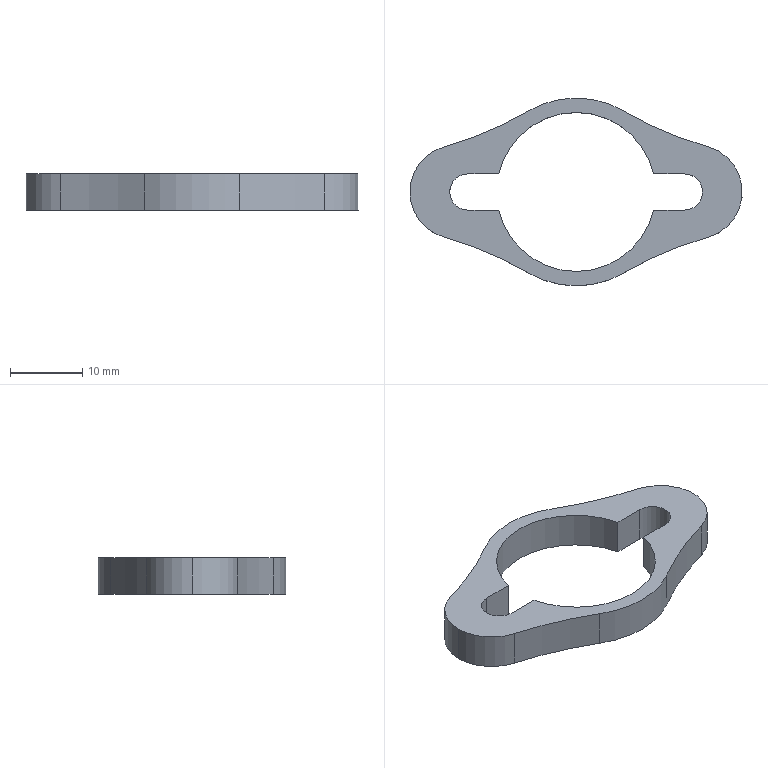Part | SolidWorks | features BaseBody 1 | 1 solid | 20 faces | box 46 x 26 x 5 mm | volume 1841 mm3 | cylinder 14 | plane 6 | commonest cylinder face diameters 100 x4 5 x3 13 x3 22 x2 26 x2
STEP:
#1=CARTESIAN_POINT('',(465.537,40.215,0.366));
#2=VERTEX_POINT('',#1);
#3=CARTESIAN_POINT('',(463.037,37.715,0.366));
#4=VERTEX_POINT('',#3);
#5=CARTESIAN_POINT('',(465.537,37.715,0.366));
#6=DIRECTION('',(-0.000000013,0.,1.));
#7=DIRECTION('',(-1.,0.,-0.000000013));
#8=AXIS2_PLACEMENT_3D('',#5,#6,#7);
#9=CIRCLE('',#8,2.5);
#10=EDGE_CURVE('',#2,#4,#9,.T.);
#11=ORIENTED_EDGE('',*,*,#10,.T.);
#12=CARTESIAN_POINT('',(463.037,37.715,-4.634));
#13=VERTEX_POINT('',#12);
#14=CARTESIAN_POINT('',(463.037,37.715,0.366));
#15=DIRECTION('',(0.000000013,0.,-1.));
#16=VECTOR('',#15,1000.);
#17=LINE('',#14,#16);
#18=EDGE_CURVE('',#4,#13,#17,.T.);
#19=ORIENTED_EDGE('',*,*,#18,.T.);
#20=CARTESIAN_POINT('',(465.537,40.215,-4.634));
#21=VERTEX_POINT('',#20);
#22=CARTESIAN_POINT('',(465.537,37.715,-4.634));
#23=DIRECTION('',(0.000000013,0.,-1.));
#24=DIRECTION('',(-1.,0.,-0.000000013));
#25=AXIS2_PLACEMENT_3D('',#22,#23,#24);
#26=CIRCLE('',#25,2.5);
#27=EDGE_CURVE('',#13,#21,#26,.T.);
#28=ORIENTED_EDGE('',*,*,#27,.T.);
#29=CARTESIAN_POINT('',(465.537,40.215,-2.134));
#30=DIRECTION('',(0.000000013,0.,-1.));
#31=VECTOR('',#30,1000.);
#32=LINE('',#29,#31);
#33=EDGE_CURVE('',#2,#21,#32,.T.);
#34=ORIENTED_EDGE('',*,*,#33,.F.);
#35=EDGE_LOOP('',(#11,#19,#28,#34));
#36=FACE_OUTER_BOUND('',#35,.T.);
#37=CARTESIAN_POINT('',(465.537,37.715,0.366));
#38=DIRECTION('',(0.000000013,0.,-1.));
#39=DIRECTION('',(-1.,0.,-0.000000013));
#40=AXIS2_PLACEMENT_3D('',#37,#38,#39);
#41=CYLINDRICAL_SURFACE('',#40,2.5);
#42=ADVANCED_FACE('',(#36),#41,.F.);
#43=CARTESIAN_POINT('',(462.278,31.457,0.366));
#44=VERTEX_POINT('',#43);
#45=CARTESIAN_POINT('',(457.537,37.715,0.366));
#46=VERTEX_POINT('',#45);
#47=CARTESIAN_POINT('',(464.037,37.715,0.366));
#48=DIRECTION('',(0.000000013,0.,-1.));
#49=DIRECTION('',(-1.,0.,-0.000000013));
#50=AXIS2_PLACEMENT_3D('',#47,#48,#49);
#51=CIRCLE('',#50,6.5);
#52=EDGE_CURVE('',#44,#46,#51,.T.);
#53=ORIENTED_EDGE('',*,*,#52,.T.);
#54=CARTESIAN_POINT('',(457.537,37.715,-4.634));
#55=VERTEX_POINT('',#54);
#56=CARTESIAN_POINT('',(457.537,37.715,0.366));
#57=DIRECTION('',(0.000000013,0.,-1.));
#58=VECTOR('',#57,1000.);
#59=LINE('',#56,#58);
#60=EDGE_CURVE('',#46,#55,#59,.T.);
#61=ORIENTED_EDGE('',*,*,#60,.T.);
#62=CARTESIAN_POINT('',(462.278,31.457,-4.634));
#63=VERTEX_POINT('',#62);
#64=CARTESIAN_POINT('',(464.037,37.715,-4.634));
#65=DIRECTION('',(0.000000013,0.,-1.));
#66=DIRECTION('',(-1.,0.,-0.000000013));
#67=AXIS2_PLACEMENT_3D('',#64,#65,#66);
#68=CIRCLE('',#67,6.5);
#69=EDGE_CURVE('',#63,#55,#68,.T.);
#70=ORIENTED_EDGE('',*,*,#69,.F.);
#71=CARTESIAN_POINT('',(462.278,31.457,-2.134));
#72=DIRECTION('',(0.000000013,0.,-1.));
#73=VECTOR('',#72,1000.);
#74=LINE('',#71,#73);
#75=EDGE_CURVE('',#44,#63,#74,.T.);
#76=ORIENTED_EDGE('',*,*,#75,.F.);
#77=EDGE_LOOP('',(#53,#61,#70,#76));
#78=FACE_OUTER_BOUND('',#77,.T.);
#79=CARTESIAN_POINT('',(464.037,37.715,0.366));
#80=DIRECTION('',(0.000000013,0.,-1.));
#81=DIRECTION('',(-1.,0.,-0.000000013));
#82=AXIS2_PLACEMENT_3D('',#79,#80,#81);
#83=CYLINDRICAL_SURFACE('',#82,6.5);
#84=ADVANCED_FACE('',(#78),#83,.T.);
#85=CARTESIAN_POINT('',(491.249,40.215,0.366));
#86=VERTEX_POINT('',#85);
#87=CARTESIAN_POINT('',(469.825,40.215,0.366));
#88=VERTEX_POINT('',#87);
#89=CARTESIAN_POINT('',(480.537,37.715,0.366));
#90=DIRECTION('',(-0.000000013,0.,1.));
#91=DIRECTION('',(-1.,0.,-0.000000013));
#92=AXIS2_PLACEMENT_3D('',#89,#90,#91);
#93=CIRCLE('',#92,11.);
#94=EDGE_CURVE('',#86,#88,#93,.T.);
#95=ORIENTED_EDGE('',*,*,#94,.F.);
#96=CARTESIAN_POINT('',(495.537,40.215,0.366));
#97=VERTEX_POINT('',#96);
#98=CARTESIAN_POINT('',(480.537,40.215,0.366));
#99=DIRECTION('',(-1.,0.,-0.000000013));
#100=VECTOR('',#99,1000.);
#101=LINE('',#98,#100);
#102=EDGE_CURVE('',#97,#86,#101,.T.);
#103=ORIENTED_EDGE('',*,*,#102,.F.);
#104=CARTESIAN_POINT('',(495.537,35.215,0.366));
#105=VERTEX_POINT('',#104);
#106=CARTESIAN_POINT('',(495.537,37.715,0.366));
#107=DIRECTION('',(-0.000000013,0.,1.));
#108=DIRECTION('',(-1.,0.,-0.000000013));
#109=AXIS2_PLACEMENT_3D('',#106,#107,#108);
#110=CIRCLE('',#109,2.5);
#111=EDGE_CURVE('',#105,#97,#110,.T.);
#112=ORIENTED_EDGE('',*,*,#111,.F.);
#113=CARTESIAN_POINT('',(491.249,35.215,0.366));
#114=VERTEX_POINT('',#113);
#115=CARTESIAN_POINT('',(480.537,35.215,0.366));
#116=DIRECTION('',(1.,0.,0.000000013));
#117=VECTOR('',#116,1000.);
#118=LINE('',#115,#117);
#119=EDGE_CURVE('',#114,#105,#118,.T.);
#120=ORIENTED_EDGE('',*,*,#119,.F.);
#121=CARTESIAN_POINT('',(469.825,35.215,0.366));
#122=VERTEX_POINT('',#121);
#123=CARTESIAN_POINT('',(480.537,37.715,0.366));
#124=DIRECTION('',(-0.000000013,0.,1.));
#125=DIRECTION('',(-1.,0.,-0.000000013));
#126=AXIS2_PLACEMENT_3D('',#123,#124,#125);
#127=CIRCLE('',#126,11.);
#128=EDGE_CURVE('',#122,#114,#127,.T.);
#129=ORIENTED_EDGE('',*,*,#128,.F.);
#130=CARTESIAN_POINT('',(465.537,35.215,0.366));
#131=VERTEX_POINT('',#130);
#132=CARTESIAN_POINT('',(480.537,35.215,0.366));
#133=DIRECTION('',(1.,0.,0.000000013));
#134=VECTOR('',#133,1000.);
#135=LINE('',#132,#134);
#136=EDGE_CURVE('',#131,#122,#135,.T.);
#137=ORIENTED_EDGE('',*,*,#136,.F.);
#138=CARTESIAN_POINT('',(465.537,37.715,0.366));
#139=DIRECTION('',(-0.000000013,0.,1.));
#140=DIRECTION('',(-1.,0.,-0.000000013));
#141=AXIS2_PLACEMENT_3D('',#138,#139,#140);
#142=CIRCLE('',#141,2.5);
#143=EDGE_CURVE('',#4,#131,#142,.T.);
#144=ORIENTED_EDGE('',*,*,#143,.F.);
#145=ORIENTED_EDGE('',*,*,#10,.F.);
#146=CARTESIAN_POINT('',(480.537,40.215,0.366));
#147=DIRECTION('',(-1.,0.,-0.000000013));
#148=VECTOR('',#147,1000.);
#149=LINE('',#146,#148);
#150=EDGE_CURVE('',#88,#2,#149,.T.);
#151=ORIENTED_EDGE('',*,*,#150,.F.);
#152=EDGE_LOOP('',(#95,#103,#112,#120,#129,#137,#144,#145,#151));
#153=FACE_BOUND('',#152,.T.);
#154=CARTESIAN_POINT('',(462.278,43.972,0.366));
#155=VERTEX_POINT('',#154);
#156=CARTESIAN_POINT('',(473.977,48.939,0.366));
#157=VERTEX_POINT('',#156);
#158=CARTESIAN_POINT('',(448.749,92.107,0.366));
#159=DIRECTION('',(-0.000000013,0.,1.));
#160=DIRECTION('',(-1.,0.,-0.000000013));
#161=AXIS2_PLACEMENT_3D('',#158,#159,#160);
#162=CIRCLE('',#161,50.);
#163=EDGE_CURVE('',#155,#157,#162,.T.);
#164=ORIENTED_EDGE('',*,*,#163,.F.);
#165=CARTESIAN_POINT('',(464.037,37.715,0.366));
#166=DIRECTION('',(0.000000013,0.,-1.));
#167=DIRECTION('',(-1.,0.,-0.000000013));
#168=AXIS2_PLACEMENT_3D('',#165,#166,#167);
#169=CIRCLE('',#168,6.5);
#170=EDGE_CURVE('',#46,#155,#169,.T.);
#171=ORIENTED_EDGE('',*,*,#170,.F.);
#172=ORIENTED_EDGE('',*,*,#52,.F.);
#173=CARTESIAN_POINT('',(473.977,26.491,0.366));
#174=VERTEX_POINT('',#173);
#175=CARTESIAN_POINT('',(448.749,-16.678,0.366));
#176=DIRECTION('',(-0.000000013,0.,1.));
#177=DIRECTION('',(-1.,0.,-0.000000013));
#178=AXIS2_PLACEMENT_3D('',#175,#176,#177);
#179=CIRCLE('',#178,50.);
#180=EDGE_CURVE('',#174,#44,#179,.T.);
#181=ORIENTED_EDGE('',*,*,#180,.F.);
#182=CARTESIAN_POINT('',(487.096,26.491,0.366));
#183=VERTEX_POINT('',#182);
#184=CARTESIAN_POINT('',(480.537,37.715,0.366));
#185=DIRECTION('',(0.000000013,0.,-1.));
#186=DIRECTION('',(-1.,0.,-0.000000013));
#187=AXIS2_PLACEMENT_3D('',#184,#185,#186);
#188=CIRCLE('',#187,13.);
#189=EDGE_CURVE('',#183,#174,#188,.T.);
#190=ORIENTED_EDGE('',*,*,#189,.F.);
#191=CARTESIAN_POINT('',(498.796,31.457,0.366));
#192=VERTEX_POINT('',#191);
#193=CARTESIAN_POINT('',(512.325,-16.678,0.366));
#194=DIRECTION('',(-0.000000013,0.,1.));
#195=DIRECTION('',(-1.,0.,-0.000000013));
#196=AXIS2_PLACEMENT_3D('',#193,#194,#195);
#197=CIRCLE('',#196,50.);
#198=EDGE_CURVE('',#192,#183,#197,.T.);
#199=ORIENTED_EDGE('',*,*,#198,.F.);
#200=CARTESIAN_POINT('',(498.796,43.972,0.366));
#201=VERTEX_POINT('',#200);
#202=CARTESIAN_POINT('',(497.037,37.715,0.366));
#203=DIRECTION('',(0.000000013,0.,-1.));
#204=DIRECTION('',(-1.,0.,-0.000000013));
#205=AXIS2_PLACEMENT_3D('',#202,#203,#204);
#206=CIRCLE('',#205,6.5);
#207=EDGE_CURVE('',#201,#192,#206,.T.);
#208=ORIENTED_EDGE('',*,*,#207,.F.);
#209=CARTESIAN_POINT('',(487.096,48.939,0.366));
#210=VERTEX_POINT('',#209);
#211=CARTESIAN_POINT('',(512.325,92.107,0.366));
#212=DIRECTION('',(-0.000000013,0.,1.));
#213=DIRECTION('',(-1.,0.,-0.000000013));
#214=AXIS2_PLACEMENT_3D('',#211,#212,#213);
#215=CIRCLE('',#214,50.);
#216=EDGE_CURVE('',#210,#201,#215,.T.);
#217=ORIENTED_EDGE('',*,*,#216,.F.);
#218=CARTESIAN_POINT('',(480.537,37.715,0.366));
#219=DIRECTION('',(0.000000013,0.,-1.));
#220=DIRECTION('',(-1.,0.,-0.000000013));
#221=AXIS2_PLACEMENT_3D('',#218,#219,#220);
#222=CIRCLE('',#221,13.);
#223=EDGE_CURVE('',#157,#210,#222,.T.);
#224=ORIENTED_EDGE('',*,*,#223,.F.);
#225=EDGE_LOOP('',(#164,#171,#172,#181,#190,#199,#208,#217,#224));
#226=FACE_OUTER_BOUND('',#225,.T.);
#227=CARTESIAN_POINT('',(504.464,24.183,0.366));
#228=DIRECTION('',(0.000000013,0.,-1.));
#229=DIRECTION('',(-1.,0.,-0.000000013));
#230=AXIS2_PLACEMENT_3D('',#227,#228,#229);
#231=PLANE('',#230);
#232=ADVANCED_FACE('',(#153,#226),#231,.F.);
#233=CARTESIAN_POINT('',(469.825,40.215,-4.634));
#234=VERTEX_POINT('',#233);
#235=CARTESIAN_POINT('',(467.681,40.215,-4.634));
#236=DIRECTION('',(1.,0.,0.000000013));
#237=VECTOR('',#236,1000.);
#238=LINE('',#235,#237);
#239=EDGE_CURVE('',#21,#234,#238,.T.);
#240=ORIENTED_EDGE('',*,*,#239,.T.);
#241=CARTESIAN_POINT('',(469.825,40.215,-2.134));
#242=DIRECTION('',(-0.000000013,0.,1.));
#243=VECTOR('',#242,1000.);
#244=LINE('',#241,#243);
#245=EDGE_CURVE('',#234,#88,#244,.T.);
#246=ORIENTED_EDGE('',*,*,#245,.T.);
#247=ORIENTED_EDGE('',*,*,#150,.T.);
#248=ORIENTED_EDGE('',*,*,#33,.T.);
#249=EDGE_LOOP('',(#240,#246,#247,#248));
#250=FACE_OUTER_BOUND('',#249,.T.);
#251=CARTESIAN_POINT('',(469.91,40.215,0.466));
#252=DIRECTION('',(0.,-1.,0.));
#253=DIRECTION('',(-1.,0.,-0.000000013));
#254=AXIS2_PLACEMENT_3D('',#251,#252,#253);
#255=PLANE('',#254);
#256=ADVANCED_FACE('',(#250),#255,.T.);
#257=CARTESIAN_POINT('',(491.249,40.215,-4.634));
#258=VERTEX_POINT('',#257);
#259=CARTESIAN_POINT('',(480.537,37.715,-4.634));
#260=DIRECTION('',(0.000000013,0.,-1.));
#261=DIRECTION('',(-1.,0.,-0.000000013));
#262=AXIS2_PLACEMENT_3D('',#259,#260,#261);
#263=CIRCLE('',#262,11.);
#264=EDGE_CURVE('',#234,#258,#263,.T.);
#265=ORIENTED_EDGE('',*,*,#264,.T.);
#266=CARTESIAN_POINT('',(491.249,40.215,-2.134));
#267=DIRECTION('',(-0.000000013,0.,1.));
#268=VECTOR('',#267,1000.);
#269=LINE('',#266,#268);
#270=EDGE_CURVE('',#258,#86,#269,.T.);
#271=ORIENTED_EDGE('',*,*,#270,.T.);
#272=ORIENTED_EDGE('',*,*,#94,.T.);
#273=ORIENTED_EDGE('',*,*,#245,.F.);
#274=EDGE_LOOP('',(#265,#271,#272,#273));
#275=FACE_OUTER_BOUND('',#274,.T.);
#276=CARTESIAN_POINT('',(480.537,37.715,0.366));
#277=DIRECTION('',(0.000000013,0.,-1.));
#278=DIRECTION('',(-1.,0.,-0.000000013));
#279=AXIS2_PLACEMENT_3D('',#276,#277,#278);
#280=CYLINDRICAL_SURFACE('',#279,11.);
#281=ADVANCED_FACE('',(#275),#280,.F.);
#282=CARTESIAN_POINT('',(495.537,40.215,-4.634));
#283=VERTEX_POINT('',#282);
#284=CARTESIAN_POINT('',(493.393,40.215,-4.634));
#285=DIRECTION('',(1.,0.,0.000000013));
#286=VECTOR('',#285,1000.);
#287=LINE('',#284,#286);
#288=EDGE_CURVE('',#258,#283,#287,.T.);
#289=ORIENTED_EDGE('',*,*,#288,.T.);
#290=CARTESIAN_POINT('',(495.537,40.215,-2.134));
#291=DIRECTION('',(-0.000000013,0.,1.));
#292=VECTOR('',#291,1000.);
#293=LINE('',#290,#292);
#294=EDGE_CURVE('',#283,#97,#293,.T.);
#295=ORIENTED_EDGE('',*,*,#294,.T.);
#296=ORIENTED_EDGE('',*,*,#102,.T.);
#297=ORIENTED_EDGE('',*,*,#270,.F.);
#298=EDGE_LOOP('',(#289,#295,#296,#297));
#299=FACE_OUTER_BOUND('',#298,.T.);
#300=CARTESIAN_POINT('',(495.623,40.215,0.466));
#301=DIRECTION('',(0.,-1.,0.));
#302=DIRECTION('',(-1.,0.,-0.000000013));
#303=AXIS2_PLACEMENT_3D('',#300,#301,#302);
#304=PLANE('',#303);
#305=ADVANCED_FACE('',(#299),#304,.T.);
#306=ORIENTED_EDGE('',*,*,#294,.F.);
#307=CARTESIAN_POINT('',(495.537,35.215,-4.634));
#308=VERTEX_POINT('',#307);
#309=CARTESIAN_POINT('',(495.537,37.715,-4.634));
#310=DIRECTION('',(0.000000013,0.,-1.));
#311=DIRECTION('',(-1.,0.,-0.000000013));
#312=AXIS2_PLACEMENT_3D('',#309,#310,#311);
#313=CIRCLE('',#312,2.5);
#314=EDGE_CURVE('',#283,#308,#313,.T.);
#315=ORIENTED_EDGE('',*,*,#314,.T.);
#316=CARTESIAN_POINT('',(495.537,35.215,-2.134));
#317=DIRECTION('',(-0.000000013,0.,1.));
#318=VECTOR('',#317,1000.);
#319=LINE('',#316,#318);
#320=EDGE_CURVE('',#308,#105,#319,.T.);
#321=ORIENTED_EDGE('',*,*,#320,.T.);
#322=ORIENTED_EDGE('',*,*,#111,.T.);
#323=EDGE_LOOP('',(#306,#315,#321,#322));
#324=FACE_OUTER_BOUND('',#323,.T.);
#325=CARTESIAN_POINT('',(495.537,37.715,0.366));
#326=DIRECTION('',(0.000000013,0.,-1.));
#327=DIRECTION('',(-1.,0.,-0.000000013));
#328=AXIS2_PLACEMENT_3D('',#325,#326,#327);
#329=CYLINDRICAL_SURFACE('',#328,2.5);
#330=ADVANCED_FACE('',(#324),#329,.F.);
#331=CARTESIAN_POINT('',(491.249,35.215,-4.634));
#332=VERTEX_POINT('',#331);
#333=CARTESIAN_POINT('',(493.393,35.215,-4.634));
#334=DIRECTION('',(-1.,0.,-0.000000013));
#335=VECTOR('',#334,1000.);
#336=LINE('',#333,#335);
#337=EDGE_CURVE('',#308,#332,#336,.T.);
#338=ORIENTED_EDGE('',*,*,#337,.T.);
#339=CARTESIAN_POINT('',(491.249,35.215,-2.134));
#340=DIRECTION('',(-0.000000013,0.,1.));
#341=VECTOR('',#340,1000.);
#342=LINE('',#339,#341);
#343=EDGE_CURVE('',#332,#114,#342,.T.);
#344=ORIENTED_EDGE('',*,*,#343,.T.);
#345=ORIENTED_EDGE('',*,*,#119,.T.);
#346=ORIENTED_EDGE('',*,*,#320,.F.);
#347=EDGE_LOOP('',(#338,#344,#345,#346));
#348=FACE_OUTER_BOUND('',#347,.T.);
#349=CARTESIAN_POINT('',(491.163,35.215,0.466));
#350=DIRECTION('',(0.,1.,0.));
#351=DIRECTION('',(1.,0.,0.000000013));
#352=AXIS2_PLACEMENT_3D('',#349,#350,#351);
#353=PLANE('',#352);
#354=ADVANCED_FACE('',(#348),#353,.T.);
#355=CARTESIAN_POINT('',(469.825,35.215,-4.634));
#356=VERTEX_POINT('',#355);
#357=CARTESIAN_POINT('',(480.537,37.715,-4.634));
#358=DIRECTION('',(0.000000013,0.,-1.));
#359=DIRECTION('',(-1.,0.,-0.000000013));
#360=AXIS2_PLACEMENT_3D('',#357,#358,#359);
#361=CIRCLE('',#360,11.);
#362=EDGE_CURVE('',#332,#356,#361,.T.);
#363=ORIENTED_EDGE('',*,*,#362,.T.);
#364=CARTESIAN_POINT('',(469.825,35.215,-2.134));
#365=DIRECTION('',(-0.000000013,0.,1.));
#366=VECTOR('',#365,1000.);
#367=LINE('',#364,#366);
#368=EDGE_CURVE('',#356,#122,#367,.T.);
#369=ORIENTED_EDGE('',*,*,#368,.T.);
#370=ORIENTED_EDGE('',*,*,#128,.T.);
#371=ORIENTED_EDGE('',*,*,#343,.F.);
#372=EDGE_LOOP('',(#363,#369,#370,#371));
#373=FACE_OUTER_BOUND('',#372,.T.);
#374=CARTESIAN_POINT('',(480.537,37.715,0.366));
#375=DIRECTION('',(0.000000013,0.,-1.));
#376=DIRECTION('',(-1.,0.,-0.000000013));
#377=AXIS2_PLACEMENT_3D('',#374,#375,#376);
#378=CYLINDRICAL_SURFACE('',#377,11.);
#379=ADVANCED_FACE('',(#373),#378,.F.);
#380=CARTESIAN_POINT('',(465.537,35.215,-4.634));
#381=VERTEX_POINT('',#380);
#382=CARTESIAN_POINT('',(467.681,35.215,-4.634));
#383=DIRECTION('',(-1.,0.,-0.000000013));
#384=VECTOR('',#383,1000.);
#385=LINE('',#382,#384);
#386=EDGE_CURVE('',#356,#381,#385,.T.);
#387=ORIENTED_EDGE('',*,*,#386,.T.);
#388=CARTESIAN_POINT('',(465.537,35.215,-2.134));
#389=DIRECTION('',(-0.000000013,0.,1.));
#390=VECTOR('',#389,1000.);
#391=LINE('',#388,#390);
#392=EDGE_CURVE('',#381,#131,#391,.T.);
#393=ORIENTED_EDGE('',*,*,#392,.T.);
#394=ORIENTED_EDGE('',*,*,#136,.T.);
#395=ORIENTED_EDGE('',*,*,#368,.F.);
#396=EDGE_LOOP('',(#387,#393,#394,#395));
#397=FACE_OUTER_BOUND('',#396,.T.);
#398=CARTESIAN_POINT('',(465.451,35.215,0.466));
#399=DIRECTION('',(0.,1.,0.));
#400=DIRECTION('',(1.,0.,0.000000013));
#401=AXIS2_PLACEMENT_3D('',#398,#399,#400);
#402=PLANE('',#401);
#403=ADVANCED_FACE('',(#397),#402,.T.);
#404=ORIENTED_EDGE('',*,*,#18,.F.);
#405=ORIENTED_EDGE('',*,*,#143,.T.);
#406=ORIENTED_EDGE('',*,*,#392,.F.);
#407=CARTESIAN_POINT('',(465.537,37.715,-4.634));
#408=DIRECTION('',(0.000000013,0.,-1.));
#409=DIRECTION('',(-1.,0.,-0.000000013));
#410=AXIS2_PLACEMENT_3D('',#407,#408,#409);
#411=CIRCLE('',#410,2.5);
#412=EDGE_CURVE('',#381,#13,#411,.T.);
#413=ORIENTED_EDGE('',*,*,#412,.T.);
#414=EDGE_LOOP('',(#404,#405,#406,#413));
#415=FACE_OUTER_BOUND('',#414,.T.);
#416=CARTESIAN_POINT('',(465.537,37.715,0.366));
#417=DIRECTION('',(0.000000013,0.,-1.));
#418=DIRECTION('',(-1.,0.,-0.000000013));
#419=AXIS2_PLACEMENT_3D('',#416,#417,#418);
#420=CYLINDRICAL_SURFACE('',#419,2.5);
#421=ADVANCED_FACE('',(#415),#420,.F.);
#422=CARTESIAN_POINT('',(487.096,48.939,-4.634));
#423=VERTEX_POINT('',#422);
#424=CARTESIAN_POINT('',(487.096,48.939,-2.134));
#425=DIRECTION('',(-0.000000013,0.,1.));
#426=VECTOR('',#425,1000.);
#427=LINE('',#424,#426);
#428=EDGE_CURVE('',#423,#210,#427,.T.);
#429=ORIENTED_EDGE('',*,*,#428,.F.);
#430=CARTESIAN_POINT('',(473.977,48.939,-4.634));
#431=VERTEX_POINT('',#430);
#432=CARTESIAN_POINT('',(480.537,37.715,-4.634));
#433=DIRECTION('',(0.000000013,0.,-1.));
#434=DIRECTION('',(-1.,0.,-0.000000013));
#435=AXIS2_PLACEMENT_3D('',#432,#433,#434);
#436=CIRCLE('',#435,13.);
#437=EDGE_CURVE('',#431,#423,#436,.T.);
#438=ORIENTED_EDGE('',*,*,#437,.F.);
#439=CARTESIAN_POINT('',(473.977,48.939,-2.134));
#440=DIRECTION('',(0.000000013,0.,-1.));
#441=VECTOR('',#440,1000.);
#442=LINE('',#439,#441);
#443=EDGE_CURVE('',#157,#431,#442,.T.);
#444=ORIENTED_EDGE('',*,*,#443,.F.);
#445=ORIENTED_EDGE('',*,*,#223,.T.);
#446=EDGE_LOOP('',(#429,#438,#444,#445));
#447=FACE_OUTER_BOUND('',#446,.T.);
#448=CARTESIAN_POINT('',(480.537,37.715,0.366));
#449=DIRECTION('',(0.000000013,0.,-1.));
#450=DIRECTION('',(-1.,0.,-0.000000013));
#451=AXIS2_PLACEMENT_3D('',#448,#449,#450);
#452=CYLINDRICAL_SURFACE('',#451,13.);
#453=ADVANCED_FACE('',(#447),#452,.T.);
#454=CARTESIAN_POINT('',(462.278,43.972,-4.634));
#455=VERTEX_POINT('',#454);
#456=CARTESIAN_POINT('',(462.278,43.972,-2.134));
#457=DIRECTION('',(-0.000000013,0.,1.));
#458=VECTOR('',#457,1000.);
#459=LINE('',#456,#458);
#460=EDGE_CURVE('',#455,#155,#459,.T.);
#461=ORIENTED_EDGE('',*,*,#460,.T.);
#462=ORIENTED_EDGE('',*,*,#163,.T.);
#463=ORIENTED_EDGE('',*,*,#443,.T.);
#464=CARTESIAN_POINT('',(448.749,92.107,-4.634));
#465=DIRECTION('',(0.000000013,0.,-1.));
#466=DIRECTION('',(-1.,0.,-0.000000013));
#467=AXIS2_PLACEMENT_3D('',#464,#465,#466);
#468=CIRCLE('',#467,50.);
#469=EDGE_CURVE('',#431,#455,#468,.T.);
#470=ORIENTED_EDGE('',*,*,#469,.T.);
#471=EDGE_LOOP('',(#461,#462,#463,#470));
#472=FACE_OUTER_BOUND('',#471,.T.);
#473=CARTESIAN_POINT('',(448.749,92.107,0.366));
#474=DIRECTION('',(0.000000013,0.,-1.));
#475=DIRECTION('',(-1.,0.,-0.000000013));
#476=AXIS2_PLACEMENT_3D('',#473,#474,#475);
#477=CYLINDRICAL_SURFACE('',#476,50.);
#478=ADVANCED_FACE('',(#472),#477,.F.);
#479=ORIENTED_EDGE('',*,*,#60,.F.);
#480=ORIENTED_EDGE('',*,*,#170,.T.);
#481=ORIENTED_EDGE('',*,*,#460,.F.);
#482=CARTESIAN_POINT('',(464.037,37.715,-4.634));
#483=DIRECTION('',(0.000000013,0.,-1.));
#484=DIRECTION('',(-1.,0.,-0.000000013));
#485=AXIS2_PLACEMENT_3D('',#482,#483,#484);
#486=CIRCLE('',#485,6.5);
#487=EDGE_CURVE('',#55,#455,#486,.T.);
#488=ORIENTED_EDGE('',*,*,#487,.F.);
#489=EDGE_LOOP('',(#479,#480,#481,#488));
#490=FACE_OUTER_BOUND('',#489,.T.);
#491=CARTESIAN_POINT('',(464.037,37.715,0.366));
#492=DIRECTION('',(0.000000013,0.,-1.));
#493=DIRECTION('',(-1.,0.,-0.000000013));
#494=AXIS2_PLACEMENT_3D('',#491,#492,#493);
#495=CYLINDRICAL_SURFACE('',#494,6.5);
#496=ADVANCED_FACE('',(#490),#495,.T.);
#497=CARTESIAN_POINT('',(473.977,26.491,-4.634));
#498=VERTEX_POINT('',#497);
#499=CARTESIAN_POINT('',(473.977,26.491,-2.134));
#500=DIRECTION('',(-0.000000013,0.,1.));
#501=VECTOR('',#500,1000.);
#502=LINE('',#499,#501);
#503=EDGE_CURVE('',#498,#174,#502,.T.);
#504=ORIENTED_EDGE('',*,*,#503,.T.);
#505=ORIENTED_EDGE('',*,*,#180,.T.);
#506=ORIENTED_EDGE('',*,*,#75,.T.);
#507=CARTESIAN_POINT('',(448.749,-16.678,-4.634));
#508=DIRECTION('',(0.000000013,0.,-1.));
#509=DIRECTION('',(-1.,0.,-0.000000013));
#510=AXIS2_PLACEMENT_3D('',#507,#508,#509);
#511=CIRCLE('',#510,50.);
#512=EDGE_CURVE('',#63,#498,#511,.T.);
#513=ORIENTED_EDGE('',*,*,#512,.T.);
#514=EDGE_LOOP('',(#504,#505,#506,#513));
#515=FACE_OUTER_BOUND('',#514,.T.);
#516=CARTESIAN_POINT('',(448.749,-16.678,0.366));
#517=DIRECTION('',(0.000000013,0.,-1.));
#518=DIRECTION('',(-1.,0.,-0.000000013));
#519=AXIS2_PLACEMENT_3D('',#516,#517,#518);
#520=CYLINDRICAL_SURFACE('',#519,50.);
#521=ADVANCED_FACE('',(#515),#520,.F.);
#522=ORIENTED_EDGE('',*,*,#503,.F.);
#523=CARTESIAN_POINT('',(487.096,26.491,-4.634));
#524=VERTEX_POINT('',#523);
#525=CARTESIAN_POINT('',(480.537,37.715,-4.634));
#526=DIRECTION('',(0.000000013,0.,-1.));
#527=DIRECTION('',(-1.,0.,-0.000000013));
#528=AXIS2_PLACEMENT_3D('',#525,#526,#527);
#529=CIRCLE('',#528,13.);
#530=EDGE_CURVE('',#524,#498,#529,.T.);
#531=ORIENTED_EDGE('',*,*,#530,.F.);
#532=CARTESIAN_POINT('',(487.096,26.491,-2.134));
#533=DIRECTION('',(0.000000013,0.,-1.));
#534=VECTOR('',#533,1000.);
#535=LINE('',#532,#534);
#536=EDGE_CURVE('',#183,#524,#535,.T.);
#537=ORIENTED_EDGE('',*,*,#536,.F.);
#538=ORIENTED_EDGE('',*,*,#189,.T.);
#539=EDGE_LOOP('',(#522,#531,#537,#538));
#540=FACE_OUTER_BOUND('',#539,.T.);
#541=CARTESIAN_POINT('',(480.537,37.715,0.366));
#542=DIRECTION('',(0.000000013,0.,-1.));
#543=DIRECTION('',(-1.,0.,-0.000000013));
#544=AXIS2_PLACEMENT_3D('',#541,#542,#543);
#545=CYLINDRICAL_SURFACE('',#544,13.);
#546=ADVANCED_FACE('',(#540),#545,.T.);
#547=CARTESIAN_POINT('',(498.796,31.457,-4.634));
#548=VERTEX_POINT('',#547);
#549=CARTESIAN_POINT('',(498.796,31.457,-2.134));
#550=DIRECTION('',(-0.000000013,0.,1.));
#551=VECTOR('',#550,1000.);
#552=LINE('',#549,#551);
#553=EDGE_CURVE('',#548,#192,#552,.T.);
#554=ORIENTED_EDGE('',*,*,#553,.T.);
#555=ORIENTED_EDGE('',*,*,#198,.T.);
#556=ORIENTED_EDGE('',*,*,#536,.T.);
#557=CARTESIAN_POINT('',(512.325,-16.678,-4.634));
#558=DIRECTION('',(0.000000013,0.,-1.));
#559=DIRECTION('',(-1.,0.,-0.000000013));
#560=AXIS2_PLACEMENT_3D('',#557,#558,#559);
#561=CIRCLE('',#560,50.);
#562=EDGE_CURVE('',#524,#548,#561,.T.);
#563=ORIENTED_EDGE('',*,*,#562,.T.);
#564=EDGE_LOOP('',(#554,#555,#556,#563));
#565=FACE_OUTER_BOUND('',#564,.T.);
#566=CARTESIAN_POINT('',(512.325,-16.678,0.366));
#567=DIRECTION('',(0.000000013,0.,-1.));
#568=DIRECTION('',(-1.,0.,-0.000000013));
#569=AXIS2_PLACEMENT_3D('',#566,#567,#568);
#570=CYLINDRICAL_SURFACE('',#569,50.);
#571=ADVANCED_FACE('',(#565),#570,.F.);
#572=ORIENTED_EDGE('',*,*,#207,.T.);
#573=ORIENTED_EDGE('',*,*,#553,.F.);
#574=CARTESIAN_POINT('',(498.796,43.972,-4.634));
#575=VERTEX_POINT('',#574);
#576=CARTESIAN_POINT('',(497.037,37.715,-4.634));
#577=DIRECTION('',(0.000000013,0.,-1.));
#578=DIRECTION('',(-1.,0.,-0.000000013));
#579=AXIS2_PLACEMENT_3D('',#576,#577,#578);
#580=CIRCLE('',#579,6.5);
#581=EDGE_CURVE('',#575,#548,#580,.T.);
#582=ORIENTED_EDGE('',*,*,#581,.F.);
#583=CARTESIAN_POINT('',(498.796,43.972,-2.134));
#584=DIRECTION('',(0.000000013,0.,-1.));
#585=VECTOR('',#584,1000.);
#586=LINE('',#583,#585);
#587=EDGE_CURVE('',#201,#575,#586,.T.);
#588=ORIENTED_EDGE('',*,*,#587,.F.);
#589=EDGE_LOOP('',(#572,#573,#582,#588));
#590=FACE_OUTER_BOUND('',#589,.T.);
#591=CARTESIAN_POINT('',(497.037,37.715,0.366));
#592=DIRECTION('',(0.000000013,0.,-1.));
#593=DIRECTION('',(-1.,0.,-0.000000013));
#594=AXIS2_PLACEMENT_3D('',#591,#592,#593);
#595=CYLINDRICAL_SURFACE('',#594,6.5);
#596=ADVANCED_FACE('',(#590),#595,.T.);
#597=ORIENTED_EDGE('',*,*,#428,.T.);
#598=ORIENTED_EDGE('',*,*,#216,.T.);
#599=ORIENTED_EDGE('',*,*,#587,.T.);
#600=CARTESIAN_POINT('',(512.325,92.107,-4.634));
#601=DIRECTION('',(0.000000013,0.,-1.));
#602=DIRECTION('',(-1.,0.,-0.000000013));
#603=AXIS2_PLACEMENT_3D('',#600,#601,#602);
#604=CIRCLE('',#603,50.);
#605=EDGE_CURVE('',#575,#423,#604,.T.);
#606=ORIENTED_EDGE('',*,*,#605,.T.);
#607=EDGE_LOOP('',(#597,#598,#599,#606));
#608=FACE_OUTER_BOUND('',#607,.T.);
#609=CARTESIAN_POINT('',(512.325,92.107,0.366));
#610=DIRECTION('',(0.000000013,0.,-1.));
#611=DIRECTION('',(-1.,0.,-0.000000013));
#612=AXIS2_PLACEMENT_3D('',#609,#610,#611);
#613=CYLINDRICAL_SURFACE('',#612,50.);
#614=ADVANCED_FACE('',(#608),#613,.F.);
#615=ORIENTED_EDGE('',*,*,#288,.F.);
#616=ORIENTED_EDGE('',*,*,#264,.F.);
#617=ORIENTED_EDGE('',*,*,#239,.F.);
#618=ORIENTED_EDGE('',*,*,#27,.F.);
#619=ORIENTED_EDGE('',*,*,#412,.F.);
#620=ORIENTED_EDGE('',*,*,#386,.F.);
#621=ORIENTED_EDGE('',*,*,#362,.F.);
#622=ORIENTED_EDGE('',*,*,#337,.F.);
#623=ORIENTED_EDGE('',*,*,#314,.F.);
#624=EDGE_LOOP('',(#615,#616,#617,#618,#619,#620,#621,#622,#623));
#625=FACE_BOUND('',#624,.T.);
#626=ORIENTED_EDGE('',*,*,#69,.T.);
#627=ORIENTED_EDGE('',*,*,#487,.T.);
#628=ORIENTED_EDGE('',*,*,#469,.F.);
#629=ORIENTED_EDGE('',*,*,#437,.T.);
#630=ORIENTED_EDGE('',*,*,#605,.F.);
#631=ORIENTED_EDGE('',*,*,#581,.T.);
#632=ORIENTED_EDGE('',*,*,#562,.F.);
#633=ORIENTED_EDGE('',*,*,#530,.T.);
#634=ORIENTED_EDGE('',*,*,#512,.F.);
#635=EDGE_LOOP('',(#626,#627,#628,#629,#630,#631,#632,#633,#634));
#636=FACE_OUTER_BOUND('',#635,.T.);
#637=CARTESIAN_POINT('',(504.464,24.183,-4.634));
#638=DIRECTION('',(0.000000013,0.,-1.));
#639=DIRECTION('',(-1.,0.,-0.000000013));
#640=AXIS2_PLACEMENT_3D('',#637,#638,#639);
#641=PLANE('',#640);
#642=ADVANCED_FACE('',(#625,#636),#641,.T.);
#643=CLOSED_SHELL('',(#42,#84,#232,#256,#281,#305,#330,#354,#379,#403,#421,#453,#478,#496,#521,#546,#571,#596,#614,#642));
#644=MANIFOLD_SOLID_BREP('',#643);
#645=CARTESIAN_POINT('',(0.,0.,0.));
#646=DIRECTION('',(0.,0.,1.));
#647=DIRECTION('',(1.,0.,0.));
#648=AXIS2_PLACEMENT_3D('',#645,#646,#647);
#649=(LENGTH_UNIT()NAMED_UNIT(*)SI_UNIT(.MILLI.,.METRE.));
#650=UNCERTAINTY_MEASURE_WITH_UNIT(LENGTH_MEASURE(0.00001),#649,'','');
#651=(NAMED_UNIT(*)PLANE_ANGLE_UNIT()SI_UNIT($,.RADIAN.));
#652=(NAMED_UNIT(*)SI_UNIT($,.STERADIAN.)SOLID_ANGLE_UNIT());
#653=(GEOMETRIC_REPRESENTATION_CONTEXT(3)GLOBAL_UNCERTAINTY_ASSIGNED_CONTEXT((#650))GLOBAL_UNIT_ASSIGNED_CONTEXT((#649,#651,#652))REPRESENTATION_CONTEXT('',''));
#654=ADVANCED_BREP_SHAPE_REPRESENTATION('',(#644,#648),#653);